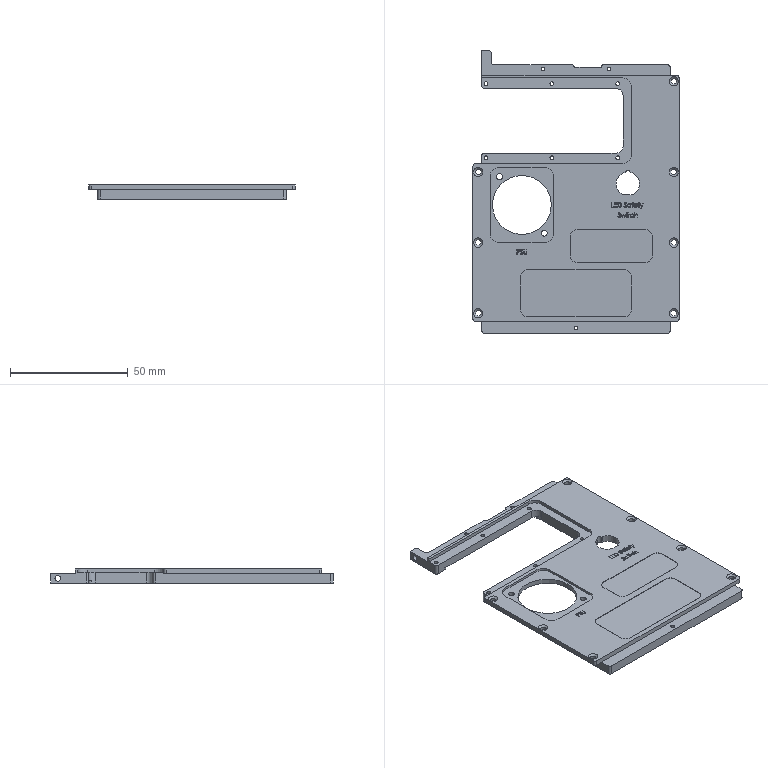CAM job | NX | 3+2 milling, drilling | part box 87.5 x 120 x 6.001 mm | stock box 92.5 x 125 x 6.001 mm
Tools:
number,name,description,diameter,corner_radius,flute_length,length,flutes
6,D1-10-D4-50-3T,D1*10*4*50-3T,1.0,0.0,10.0,11.0,3
3,D2-6-D4-50-3T-ROUGH,D2-6-D4-50-3T-粗,2.0,0.0,6.0,7.0,2
4,D2-6-D4-50-3T-FINISH,D2-6-D4-50-3T-精,2.0,0.0,6.0,7.0,3
20,D3-12-D3-75-3T,D3-12-D3-75-3T,3.0,0.0,12.0,50.0,3
2,D6-18-D6-50-3T-ROUGH,D6-18-D6-50-3T-粗,6.0,0.0,18.0,50.0,2
5,D6-18-D6-50-3T-FINISH,D6-18-D6-50-3T,6.0,0.0,18.0,50.0,3
13,D12-35-D12-75波刀,D12*35*D12*75波刀,12.0,0.0,35.0,75.0,3
1,D63面刀,D63面刀,63.0,0.0,30.0,30.0,4
7,点孔D3-50-90度,点孔D3-50-90度,3.0,0.0,0.0,50.0,2
14,点孔D5-120-90度,点孔D5-120-90度,5.0,0.0,0.0,120.0,2
8,钻头D1.84-11-D3-40,钻刀D1.84-11-D3-40,1.84,0.0,11.0,12.0,2
9,钻头D2.5-35-61,钻刀D2.5-35-61,2.5,0.0,36.0,61.0,2
10,M3,Drilling Tool,3.0,0.0,35.0,50.0,4
15,Z2.4,Drilling Tool,2.4,0.0,35.0,50.0,2
18,M2,Drilling Tool,2.0,0.0,35.0,50.0,4
Operations:
program,operation,operation_type,tool,method,geometry_group,spindle_rpm,surface_speed,feed_per_tooth,feed_cut,feed_plunge,cut_length_mm,path_length_mm,cut_time_min,machine_time_min
A1,FLOOR_WALL,VolumeBased25DMillingOperation,D63面刀,METHOD,WORKPIECE_54,4500.0,890.0,0.0389,700.0,100.0,431.049,525.049,0.6158,0.6252
A2,ADAPTIVE_MILLING,CavityMilling,D6-18-D6-50-3T-ROUGH,METHOD,WORKPIECE_54,6500.0,122.0,0.2692,3500.0,100.0,6130.806,6830.128,1.739,1.809
A2,ADAPTIVE_MILLING_COPY,CavityMilling,D6-18-D6-50-3T-ROUGH,METHOD,WORKPIECE_54,6500.0,100.0,0.1178,3500.0,100.0,8556.687,8976.148,2.398,2.44
A2,PLANAR_MILL,PlanarMilling,D6-18-D6-50-3T-ROUGH,METHOD,WORKPIECE_54,5500.0,103.0,0.0727,800.0,100.0,99.289,207.589,0.1241,0.1349
A2,FLOOR_WALL_1,VolumeBased25DMillingOperation,D6-18-D6-50-3T-ROUGH,METHOD,WORKPIECE_54,6500.0,122.0,0.1923,2500.0,100.0,691.687,791.051,0.2767,0.2866
A2,PLANAR_PROFILING,PlanarMilling,D6-18-D6-50-3T-ROUGH,METHOD,WORKPIECE_54,6500.0,122.0,0.1923,2500.0,100.0,622.5,730.3,0.249,0.2598
A2,PLANAR_PROFILING_COPY,PlanarMilling,D6-18-D6-50-3T-ROUGH,METHOD,WORKPIECE_54,6500.0,122.0,0.1923,2500.0,100.0,452.5,560.3,0.181,0.1918
A3,CAVITY_MILL_1,CavityMilling,D3-12-D3-75-3T,METHOD,WORKPIECE_54,6500.0,61.0,0.1333,2600.0,100.0,1903.314,2094.486,0.732,0.7512
A3,ZLEVEL_PROFILE_STEEP,ZLevelMilling,D2-6-D4-50-3T-ROUGH,METHOD,WORKPIECE_54,6500.0,40.0,0.1154,1500.0,100.0,2140.906,3963.246,1.427,1.609
A3,ZLEVEL_PROFILE_STEEP_COPY,ZLevelMilling,D2-6-D4-50-3T-ROUGH,METHOD,WORKPIECE_54,6500.0,40.0,0.1154,1500.0,100.0,1171.125,1647.28,0.7808,0.8284
A3,PLANAR_MILL_COPY,PlanarMilling,D2-6-D4-50-3T-ROUGH,METHOD,WORKPIECE_54,6500.0,40.0,0.1154,1500.0,100.0,134.198,242.499,0.0895,0.1003
A4,CAVITY_MILL,CavityMilling,D2-6-D4-50-3T-FINISH,METHOD,WORKPIECE_54,5500.0,34.0,0.0242,400.0,100.0,338.613,443.613,0.8465,0.857
A4,PLANAR_MILL_9,PlanarMilling,D2-6-D4-50-3T-FINISH,METHOD,WORKPIECE_54,5500.0,34.0,0.0242,400.0,100.0,170.274,270.264,0.4257,0.4357
A4,PLANAR_MILL_1,PlanarMilling,D2-6-D4-50-3T-FINISH,METHOD,WORKPIECE_54,5500.0,34.0,0.0242,400.0,100.0,759.392,1120.87,1.899,1.935
A4,PLANAR_MILL_COPY_COPY,PlanarMilling,D2-6-D4-50-3T-FINISH,METHOD,WORKPIECE_54,5500.0,34.0,0.0242,400.0,100.0,34.647,141.247,0.0866,0.0973
A4,PLANAR_MILL_COPY_COPY_COPY,PlanarMilling,D2-6-D4-50-3T-FINISH,METHOD,WORKPIECE_54,5500.0,34.0,0.0242,400.0,100.0,12.533,108.513,0.0313,0.0409
A4,PLANAR_MILL_COPY_COPY_COPY_COPY,PlanarMilling,D2-6-D4-50-3T-FINISH,METHOD,WORKPIECE_54,5500.0,34.0,0.0242,400.0,100.0,12.431,108.411,0.0311,0.0407
A4,PLANAR_MILL_COPY_COPY_COPY_COPY_COPY,PlanarMilling,D2-6-D4-50-3T-FINISH,METHOD,WORKPIECE_54,5500.0,34.0,0.0242,400.0,100.0,27.406,232.966,0.0685,0.0891
A4,PLANAR_MILL_COPY_COPY_COPY_COPY_COPY_COPY,PlanarMilling,D2-6-D4-50-3T-FINISH,METHOD,WORKPIECE_54,5500.0,34.0,0.0242,400.0,100.0,20.482,122.662,0.0512,0.0614
A4,PLANAR_MILL_6,PlanarMilling,D2-6-D4-50-3T-FINISH,METHOD,WORKPIECE_54,5500.0,17.0,0.0182,300.0,100.0,14.942,138.665,0.0498,0.0622
A4,PLANAR_MILL_6_COPY,PlanarMilling,D2-6-D4-50-3T-FINISH,METHOD,WORKPIECE_54,5500.0,17.0,0.0182,300.0,100.0,17.022,127.001,0.0567,0.0677
A5,PLANAR_MILL_COPY_COPY_COPY_COPY_COPY_COPY_COPY,PlanarMilling,D1-10-D4-50-3T,METHOD,WORKPIECE_54,5500.0,17.0,0.0182,300.0,100.0,68.235,196.541,0.2275,0.2403
A5,PLANAR_MILL_COPY_COPY_COPY_1,PlanarMilling,D1-10-D4-50-3T,METHOD,WORKPIECE_54,5500.0,17.0,0.0182,300.0,100.0,71.371,177.571,0.2379,0.2485
A6,ADAPTIVE_MILLING_COPY_COPY,CavityMilling,D6-18-D6-50-3T-FINISH,METHOD,WORKPIECE_54,5500.0,103.0,0.0424,700.0,100.0,1920.864,2716.673,2.488,2.568
A6,FLOOR_WALL_1_COPY,VolumeBased25DMillingOperation,D6-18-D6-50-3T-FINISH,METHOD,WORKPIECE_54,5500.0,103.0,0.0424,700.0,100.0,345.844,441.844,0.4941,0.5037
A6,PLANAR_MILL_2,PlanarMilling,D6-18-D6-50-3T-FINISH,METHOD,WORKPIECE_54,5500.0,103.0,0.0424,700.0,100.0,378.633,484.633,0.5409,0.5515
A6,PLANAR_MILL_2_COPY,PlanarMilling,D6-18-D6-50-3T-FINISH,METHOD,WORKPIECE_54,5500.0,103.0,0.0424,700.0,100.0,164.637,274.837,0.2352,0.2462
A6,PLANAR_MILL_2_COPY_COPY,PlanarMilling,D6-18-D6-50-3T-FINISH,METHOD,WORKPIECE_54,5500.0,103.0,0.0424,700.0,100.0,112.5,222.7,0.1607,0.1717
A6,PLANAR_MILL_2_COPY_COPY_COPY,PlanarMilling,D6-18-D6-50-3T-FINISH,METHOD,WORKPIECE_54,5500.0,103.0,0.0424,700.0,100.0,75.0,185.2,0.1071,0.1182
A6,PLANAR_MILL_2_COPY_COPY_COPY_COPY,PlanarMilling,D6-18-D6-50-3T-FINISH,METHOD,WORKPIECE_54,5500.0,103.0,0.0424,700.0,100.0,64.951,175.151,0.0928,0.1038
A7,SPOT_DRILLING,Operation,点孔D3-50-90度,METHOD,WORKPIECE_54,2000.0,18.0,0.0375,150.0,0.0,36.9,459.207,0.246,0.2882
A7,SPOT_DRILLING_COPY_1,Operation,点孔D3-50-90度,METHOD,WORKPIECE_54,2000.0,18.0,0.0375,150.0,0.0,9.0,157.757,0.06,0.0749
A7,PLANAR_MILL_3,PlanarMilling,点孔D3-50-90度,METHOD,WORKPIECE_54,6500.0,61.0,0.1154,1500.0,100.0,658.35,1276.645,0.4389,0.5007
A7,PLANAR_MILL_3_COPY,PlanarMilling,点孔D3-50-90度,METHOD,WORKPIECE_54,6500.0,61.0,0.1154,1500.0,100.0,432.506,528.106,0.2883,0.2979
A7,PLANAR_MILL_3_COPY_COPY,PlanarMilling,点孔D3-50-90度,METHOD,WORKPIECE_54,6500.0,61.0,0.1154,1500.0,100.0,159.861,257.461,0.1066,0.1163
A7,PLANAR_MILL_3_COPY_COPY_COPY_1,PlanarMilling,点孔D3-50-90度,METHOD,WORKPIECE_54,6500.0,61.0,0.1154,1500.0,100.0,22.868,120.468,0.0152,0.025
A7,PLANAR_MILL_3_COPY_COPY_COPY,PlanarMilling,点孔D3-50-90度,METHOD,WORKPIECE_54,6500.0,61.0,0.1154,1500.0,100.0,79.563,177.163,0.053,0.0628
A7,PLANAR_MILL_3_COPY_COPY_COPY_COPY_1,PlanarMilling,点孔D3-50-90度,METHOD,WORKPIECE_54,6500.0,61.0,0.1154,1500.0,100.0,60.258,157.858,0.0402,0.0499
A7,PLANAR_MILL_3_COPY_COPY_COPY_COPY,PlanarMilling,点孔D3-50-90度,METHOD,WORKPIECE_54,6500.0,61.0,0.1154,1500.0,100.0,61.321,156.921,0.0409,0.0504
A7,PLANAR_MILL_3_COPY_COPY_COPY_COPY_COPY,PlanarMilling,点孔D3-50-90度,METHOD,WORKPIECE_54,6500.0,61.0,0.1154,1500.0,100.0,117.296,220.897,0.0782,0.0886
A7,PLANAR_MILL_3_COPY_COPY_COPY_COPY_COPY_COPY,PlanarMilling,点孔D3-50-90度,METHOD,WORKPIECE_54,6500.0,61.0,0.1154,1500.0,100.0,79.796,183.397,0.0532,0.0636
A7,PLANAR_MILL_3_COPY_COPY_COPY_COPY_COPY_COPY_COPY,PlanarMilling,点孔D3-50-90度,METHOD,WORKPIECE_54,6500.0,61.0,0.1154,1500.0,100.0,119.229,368.595,0.0795,0.1044
A8,SPOT_DRILLING_COPY,Operation,钻头D1.84-11-D3-40,METHOD,WORKPIECE_54,2000.0,18.0,0.0375,150.0,0.0,36.0,223.985,0.24,0.2588
A8,SPOT_DRILLING_COPY_COPY_1,Operation,钻头D1.84-11-D3-40,METHOD,WORKPIECE_54,2000.0,18.0,0.0375,150.0,0.0,55.0,384.422,0.3667,0.3996
A9,SPOT_DRILLING_1,Operation,钻头D2.5-35-61,METHOD,WORKPIECE_54,2500.0,19.0,0.04,200.0,0.0,19.0,177.757,0.095,0.1109
A10,SPOT_DRILLING_COPY_COPY,Operation,M2,METHOD,WORKPIECE_54,300.0,18.0,0.0375,0.4,0.0,32.0,215.985,80.0,80.018
A10,SPOT_DRILLING_COPY_COPY_COPY,Operation,M2,METHOD,WORKPIECE_54,300.0,18.0,0.0375,0.4,0.0,45.0,364.422,112.5,112.532
A11,SPOT_DRILLING_1_COPY,Operation,M3,METHOD,WORKPIECE_54,300.0,2.0,0.0004,0.5,0.0,16.0,171.757,32.0,32.016
B1,FLOOR_WALL_2,VolumeBased25DMillingOperation,D63面刀,METHOD,WORKPIECE_55,4000.0,791.0,0.0938,1500.0,100.0,3508.395,4555.091,2.339,2.444
B1,FLOOR_WALL_2_COPY,VolumeBased25DMillingOperation,D12-35-D12-75波刀,METHOD,WORKPIECE_55,4000.0,791.0,0.0938,1500.0,100.0,1425.699,1519.639,0.9505,0.9599
B1,FLOOR_WALL_2_COPY_COPY,VolumeBased25DMillingOperation,D12-35-D12-75波刀,METHOD,WORKPIECE_55,5000.0,188.0,0.0333,500.0,100.0,1425.699,1519.699,2.851,2.861
B2,PLANAR_MILL_5,PlanarMilling,D6-18-D6-50-3T-ROUGH,METHOD,WORKPIECE_55,5500.0,103.0,0.2273,2500.0,100.0,363.71,557.514,0.1455,0.1649
B2,PLANAR_MILL_5_COPY_2,PlanarMilling,D6-18-D6-50-3T-ROUGH,METHOD,WORKPIECE_55,5500.0,103.0,0.2273,2500.0,100.0,513.232,669.99,0.2053,0.221
B3,PLANAR_MILL_5_COPY,PlanarMilling,D6-18-D6-50-3T-FINISH,METHOD,WORKPIECE_55,5464.0,103.0,0.0305,500.0,100.0,360.125,620.185,0.7203,0.7463
B3,PLANAR_MILL_5_COPY_1,PlanarMilling,D6-18-D6-50-3T-FINISH,METHOD,WORKPIECE_55,5464.0,103.0,0.0305,500.0,100.0,174.587,270.589,0.3492,0.3588
B3,PLANAR_MILL_5_COPY_2_COPY,PlanarMilling,D6-18-D6-50-3T-FINISH,METHOD,WORKPIECE_55,5464.0,103.0,0.0305,500.0,100.0,171.392,268.394,0.3428,0.3525
B4,PLANAR_MILL_4,PlanarMilling,D12-35-D12-75波刀,METHOD,WORKPIECE_55,5500.0,207.0,0.1515,2500.0,100.0,231.0,440.302,0.0924,0.1133
B4,PLANAR_MILL_4_COPY,PlanarMilling,D12-35-D12-75波刀,METHOD,WORKPIECE_55,5500.0,207.0,0.1515,2500.0,100.0,225.5,432.052,0.0902,0.1109
B4,PLANAR_MILL_4_COPY_COPY,PlanarMilling,D6-18-D6-50-3T-FINISH,METHOD,WORKPIECE_55,5500.0,207.0,0.1515,2500.0,100.0,21.0,119.002,0.0084,0.0182
B4,PLANAR_MILL_4_COPY_COPY_COPY,PlanarMilling,D6-18-D6-50-3T-FINISH,METHOD,WORKPIECE_55,5500.0,207.0,0.1515,2500.0,100.0,363.741,461.743,0.1455,0.1553
B5,SPOT_DRILLING_2,Operation,点孔D5-120-90度,METHOD,WORKPIECE_55,2500.0,39.0,0.024,120.0,0.0,28.0,409.844,0.2333,0.2715
B5,SPOT_DRILLING_2_COPY,Operation,点孔D5-120-90度,METHOD,WORKPIECE_55,2500.0,39.0,0.024,120.0,0.0,6.5,147.678,0.0542,0.0683
B6,SPOT_DRILLING_2_COPY_COPY,Operation,点孔D3-50-90度,METHOD,WORKPIECE_55,2500.0,39.0,0.024,120.0,0.0,27.18,321.196,0.2265,0.2559
B6,PLANAR_MILL_7,PlanarMilling,点孔D3-50-90度,METHOD,WORKPIECE_55,6500.0,61.0,0.1154,1500.0,100.0,519.876,615.478,0.3466,0.3561
B6,PLANAR_MILL_7_COPY_1,PlanarMilling,点孔D3-50-90度,METHOD,WORKPIECE_55,6500.0,61.0,0.1154,1500.0,100.0,153.637,252.239,0.1024,0.1123
B6,PLANAR_MILL_7_COPY,PlanarMilling,点孔D3-50-90度,METHOD,WORKPIECE_55,6500.0,61.0,0.1154,1500.0,100.0,151.444,399.24,0.101,0.1257
B6,PLANAR_MILL_7_COPY_COPY,PlanarMilling,点孔D3-50-90度,METHOD,WORKPIECE_55,6500.0,61.0,0.1154,1500.0,100.0,194.914,504.318,0.1299,0.1609
B7,PLANAR_MILL_COPY_COPY_COPY_COPY_COPY_COPY_COPY_1,PlanarMilling,D2-6-D4-50-3T-FINISH,METHOD,WORKPIECE_55,5500.0,34.0,0.0242,400.0,100.0,11.817,110.019,0.0295,0.0394
B8,SPOT_DRILLING_2_COPY_1,Operation,Z2.4,METHOD,WORKPIECE_55,2500.0,39.0,0.024,120.0,0.0,49.0,371.842,0.4083,0.4406
C1,PLANAR_MILL_8,PlanarMilling,D6-18-D6-50-3T-FINISH,METHOD,WORKPIECE_56,5000.0,94.0,0.02,300.0,100.0,20.0,121.5,0.0667,0.0768
C2,SPOT_DRILLING_3,Operation,点孔D5-120-90度,METHOD,WORKPIECE_56,2500.0,39.0,0.04,200.0,0.0,4.25,116.0,0.0213,0.0324
C3,SPOT_DRILLING_3_COPY,Operation,Z2.4,METHOD,WORKPIECE_56,2500.0,39.0,0.04,200.0,0.0,9.0,125.5,0.045,0.0566